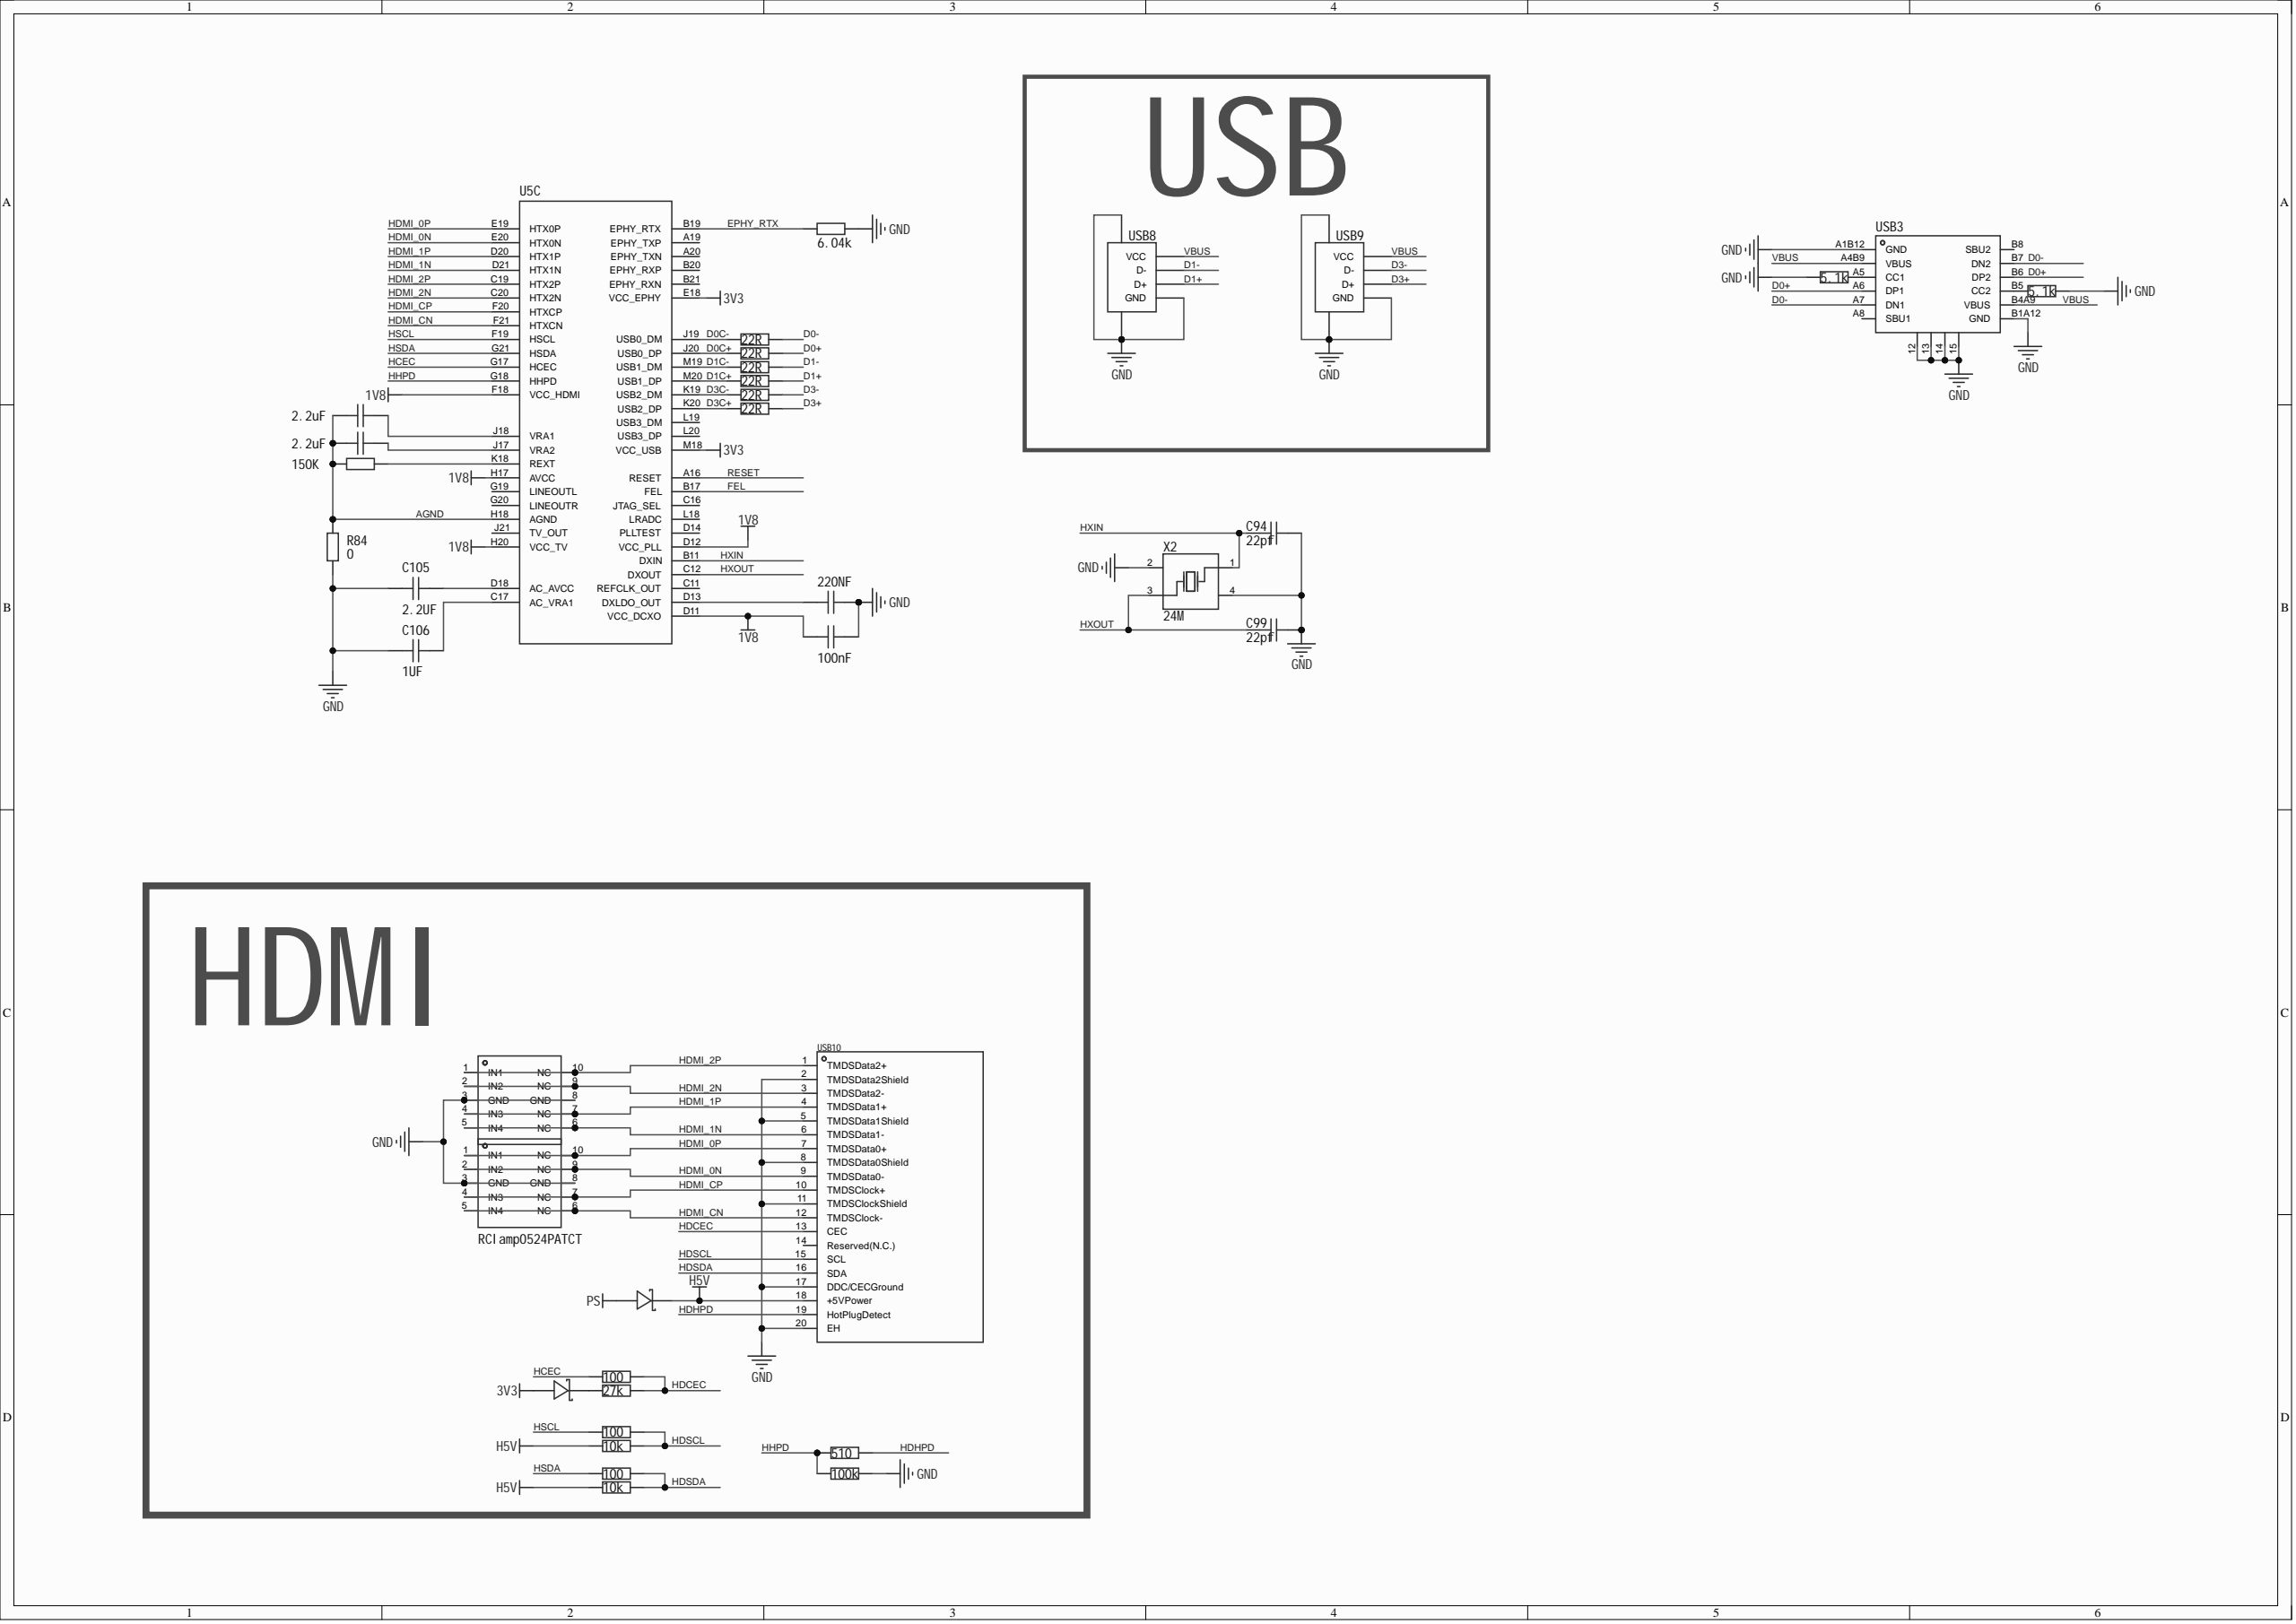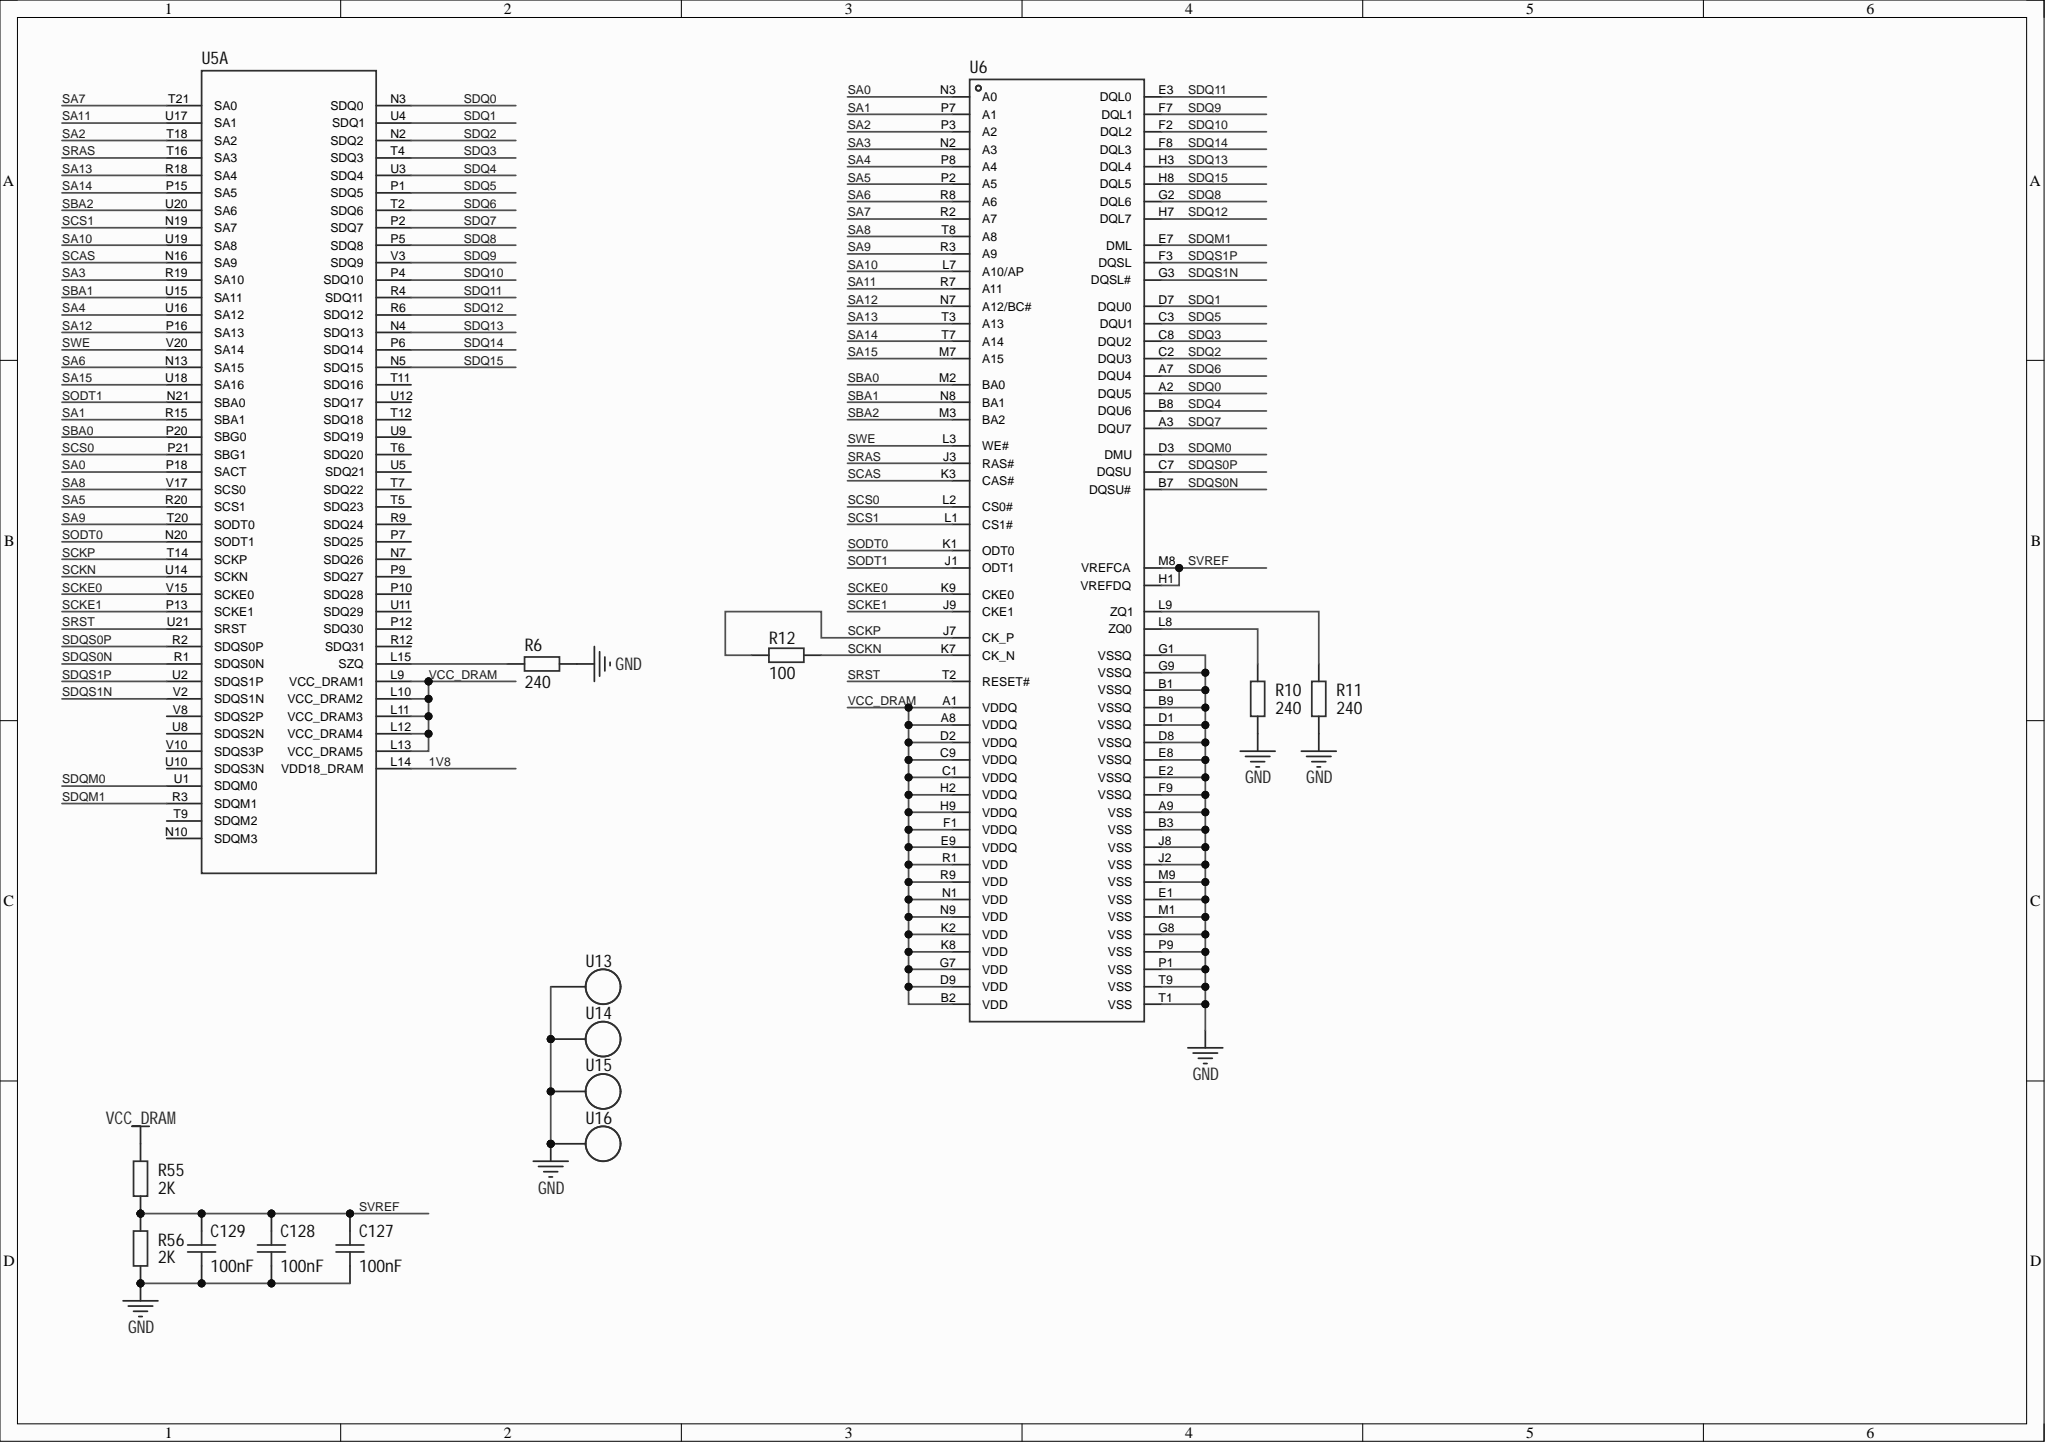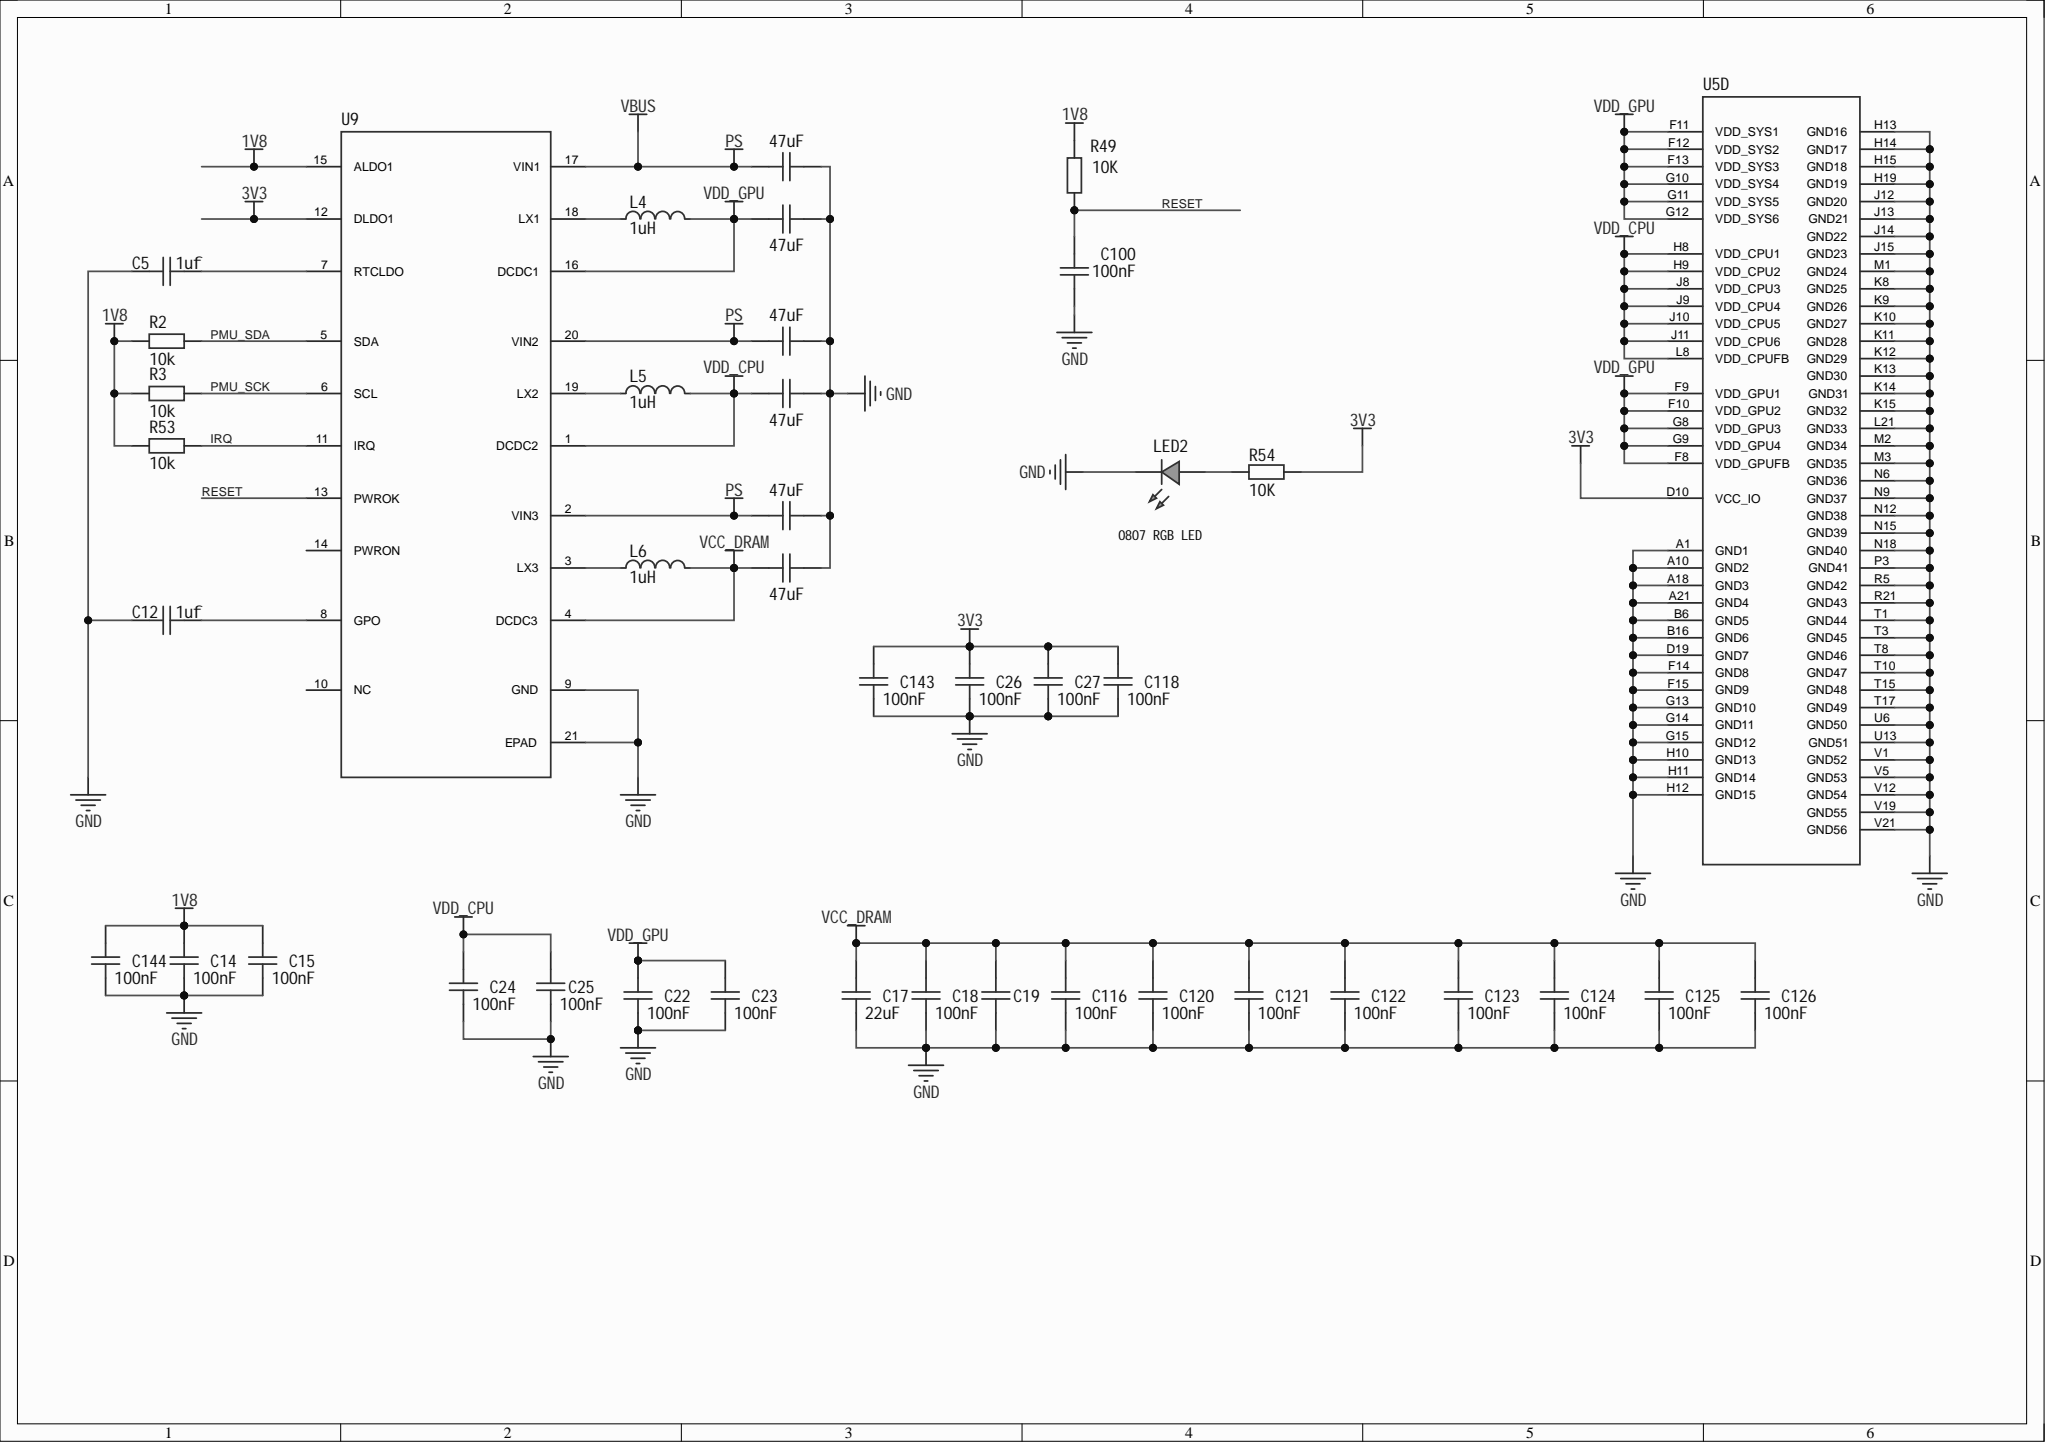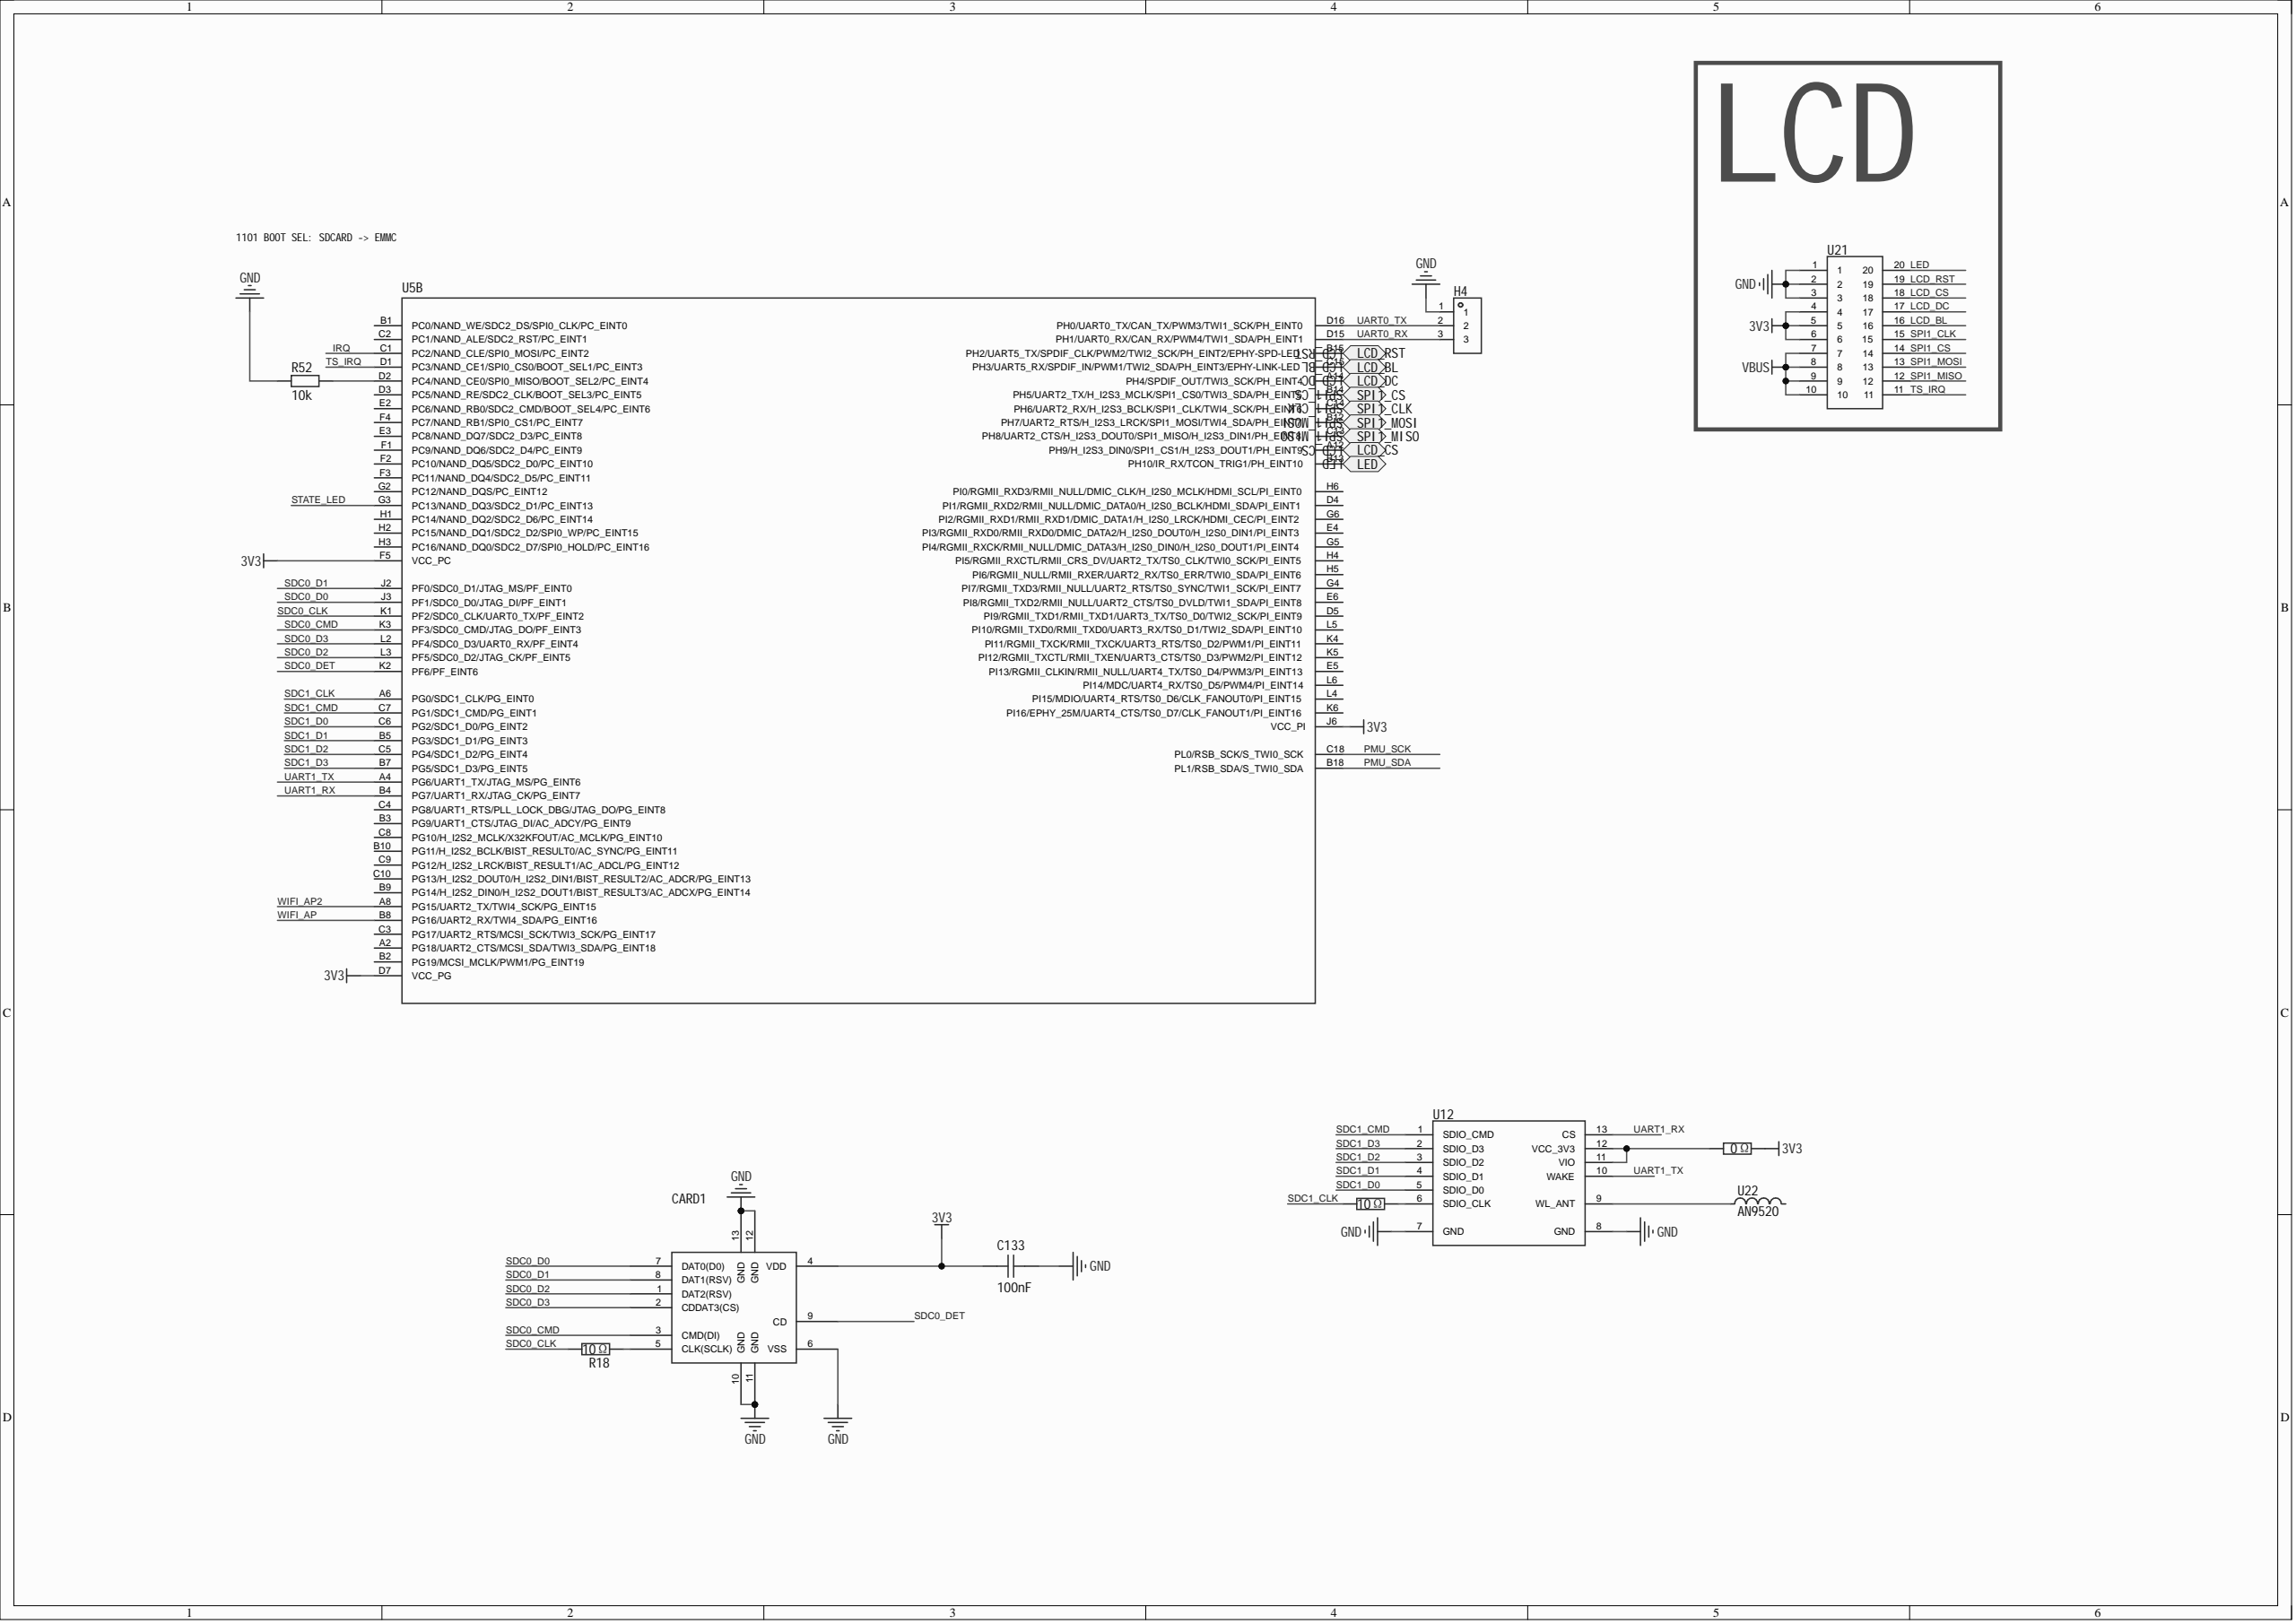Circuit board | Altium Designer | 102 parts | 149 nets
Bill of materials:
Comment,Description,Designator,Footprint,LibRef,Quantity
"","Capacitance:100nF;Tolerance:±10%;Rated voltage:16V;Temp. coefficient:X7R;","C5, C12, C14, C15, C17, C18, C19, C22, C23, C24, C25, C26, C27, C94, C99, C100, C116, C118, C120, C121, C122, C123, C124, C125, C126, C133, C143, C144","C0603 NSK","CAP_0402","28"
"2.2UF","","C105, C130, C131","C0603","CAP_0603","3"
"1UF","","C106","C0603","CAP_0603","1"
"220NF","","C108","C0603","CAP_0603","1"
"100nF","Capacitance:100nF;Tolerance:±10%;Rated voltage:50V;Material (temp. coefficient):X7R;","C127, C128, C129","C0402","CL05B104KB54PNC","3"
"100nF","","C132","C0603","CAP_0603","1"
"47uF","","C136, C137, C138, C139, C140, C141","C0805","CAP_0805","6"
"TF-015","Card connection mode:Push-push;Card type:MicroSD card (TF card);Connector type:Card socket;Body max height:-;Contact material:-;Contact plating:-;Operating temperature range:-;Soldering temperature (max):-;","CARD1","TF-SMD_TF-015","TF-015","1"
"","VBR=6V, Vc=15V, Ipp=5A","D24, D25","SLP2510P8_L2.5-W1.0-P0.50-BL","RClamp0524PATCT","2"
"","DC reverse voltage (Vr):40V;Average rectified current (Io):1A;Forward voltage drop (Vf):600mV@1A;","D26, D27","SOD-323_L1.8-W1.3-LS2.5-NSK","B5819WS","2"
"","","H4","HDR-TH_3P-P2.54-V-M","HDR-M_2.54_1x3P","1"
"1uH","Inductance:2.2uH;Tolerance:±20%;Rated current:2A;","L4, L5, L6","IND-SMD_L3.0-W3.0","SWPA3015S2R2MT","3"
"","","LED2","LED_0603","LED_0603-G","1"
"","","R2, R3, R43, R49, R52, R53, R70","R0603","Res_0402","7"
"","","R6","R0402-NSK_2","Res_0402","1"
"240","Resistor type:Thick film resistor;Resistance:200kΩ;Tolerance:±1%;Power:62.5mW;Max working voltage:50V;Temp. coefficient:±100ppm/?;","R10, R11","R0402","0402WGF2003TCE","2"
"100","Resistor type:Thick film resistor;Resistance:200kΩ;Tolerance:±1%;Power:62.5mW;Max working voltage:50V;Temp. coefficient:±100ppm/?;","R12","R0402","0402WGF2003TCE","1"
"10Ω","Tolerance:±1%;Temp. coefficient:±200ppm/;Power:1/16W;Resistance:10Ω;Max working voltage:50V;Operating temperature range:-55~+155;","R18, R86","R0603","0402WGF100JTCE","2"
"6.04k","Resistor type:Thick film resistor;Resistance:10kΩ;Tolerance:±1%;Power:100mW;","R26","R0603","0603WAF1002T5E","1"
"10K","","R54, R67, R88, R90, R117, R122","R0603","Res_0603","6"
"2K","Resistor type:Thick film resistor;Resistance:200kΩ;Tolerance:±1%;Power:62.5mW;Max working voltage:50V;Temp. coefficient:±100ppm/?;","R55, R56","R0402","0402WGF2003TCE","2"
"22R","","R66, R89, R91","R0603","Res_0603","3"
"150K","","R81","R0603","Res_0603","1"
"0","","R84","R0603","Res_0603","1"
"0Ω","Tolerance:±1%;Temp. coefficient:±200ppm/;Power:1/16W;Resistance:10Ω;Max working voltage:50V;Operating temperature range:-55~+155;","R87","R0603","0402WGF100JTCE","1"
"100","","R118, R121, R123","R0603","Res_0603","3"
"510","","R119","R0603","Res_0603","1"
"27k","","R120","R0603","Res_0603","1"
"100k","","R124","R0603","Res_0603","1"
"","","U5","BGA284P65B1200_1400H125","Allwinner_H616","1"
"","","U6","FBGA96","H5TQ4G63EFR-RDC","1"
"AXP313A","","U9","WQFN-20_L3.0-W3.0-P0.40-BL-EP","AXP1530","1"
"","","U12","WIFI模块","RTL8189ES模块","1"
"","","U13, U14, U15, U16","M3_HOLE","M3_HOLE","4"
"","","U21","BTB2X10","BTB2X10","1"
"AN9520","","U22","ANT-SMD_L9.5-W2.1","AN9520","1"
"","","USB3","USB-C-SMD_TYPEC-304-BCP16-1","TYPEC-304-BCP16","1"
"A/F board mount, type C, 10 (first two pins without curled edge), metal shell, LCP black glue=6.8","Connector type:Type-A;Standard:USB 2.0;Gender:Female;Ports:1;Contacts:4P;Rated current - power:-;","USB8, USB9","USB-A-SMD_C42496","A/F贴板 C款10前两脚无卷边铁壳LCP黑胶=6.8","2"
"HDMI 19PIN 043","Connector type:HDMI;Gender:Female;Total pins:19P;Rows:-;Mounting:Horizontal SMD;Rated current:300mA;Operating temperature range:-55℃~+85℃;","USB10","HDMI-SMD_HDMI-19PIN-043","HDMI 19PIN 043","1"
"24M","Crystal type:-;Frequency:-;Frequency tolerance:-;Frequency stability:-;Load capacitance:-;Operating temperature:-;","X2","OSC-SMD_4P-L2.0-W1.6-BL","SX32Y024000BC1T","1"
Netlist (Protel format):
[
C5
C0603 NSK




]
[
C12
C0603 NSK




]
[
C14
C0603 NSK




]
[
C15
C0603 NSK




]
[
C17
C0603 NSK




]
[
C18
C0603 NSK




]
[
C19
C0603 NSK




]
[
C22
C0603 NSK




]
[
C23
C0603 NSK




]
[
C24
C0603 NSK




]
[
C25
C0603 NSK




]
[
C26
C0603 NSK




]
[
C27
C0603 NSK




]
[
C94
C0603 NSK




]
[
C99
C0603 NSK




]
[
C100
C0603 NSK




]
[
C105
C0603
2.2UF



]
[
C106
C0603
1UF



]
[
C108
C0603
220NF



]
[
C116
C0603 NSK




]
[
C118
C0603 NSK




]
[
C120
C0603 NSK




]
[
C121
C0603 NSK




]
[
C122
C0603 NSK




]
[
C123
C0603 NSK




]
[
C124
C0603 NSK




]
[
C125
C0603 NSK




]
[
C126
C0603 NSK




]
[
C127
C0402
100nF



]
[
C128
C0402
100nF



]
[
C129
C0402
100nF



]
[
C130
C0603
2.2uF



]
[
C131
C0603
2.2uF



]
[
C132
C0603
100nF



]
[
C133
C0603 NSK




]
[
C136
C0805
47uF



]
[
C137
C0805
47uF



]
[
C138
C0805
47uF



]
[
C139
C0805
47uF



]
[
C140
C0805
47uF



]
[
C141
C0805
47uF



]
[
C143
C0603 NSK




]
[
C144
C0603 NSK




]
[
CARD1
TF-SMD_TF-015
TF-015



]
[
D24
SLP2510P8_L2.5-W1.0-P0.50-BL




]
[
D25
SLP2510P8_L2.5-W1.0-P0.50-BL




]
[
D26
SOD-323_L1.8-W1.3-LS2.5-NSK




]
[
D27
SOD-323_L1.8-W1.3-LS2.5-NSK




]
[
H4
HDR-TH_3P-P2.54-V-M




]
[
L4
IND-SMD_L3.0-W3.0
1uH



]
[
L5
IND-SMD_L3.0-W3.0
1uH



]
[
L6
IND-SMD_L3.0-W3.0
1uH



]
[
LED2
LED_0603




]
[
R2
R0603




]
[
R3
R0603




]
[
R6
R0402-NSK_2




]
[
R10
R0402
240



]
[
R11
R0402
240



]
[
R12
R0402
100



]
[
R18
R0603
10Ω



]
[
R26
R0603
6.04k



]
[
R43
R0603




]
[
R49
R0603




]
[
R52
R0603




]
[
R53
R0603




]
[
R54
R0603
10K



]
[
R55
R0402
2K



]
[
R56
R0402
2K



]
[
R66
R0603
22R



]
[
R67
R0603
10K



]
[
R70
R0603




]
[
R81
R0603
150K



]
[
R84
R0603
0



]
[
R86
R0603
10Ω



]
[
R87
R0603
0Ω



]
[
R88
R0603
10K



]
[
R89
R0603
22R



]
[
R90
R0603
10K



]
[
R91
R0603
22R



]
[
R117
R0603
10k



]
[
R118
R0603
100



]
[
R119
R0603
510



]
[
R120
R0603
27k



]
[
R121
R0603
100



]
[
R122
R0603
10k



]
[
R123
R0603
100



]
[
R124
R0603
100k



]
[
U5
BGA284P65B1200_1400H125




]
[
U6
FBGA96




]
[
U9
WQFN-20_L3.0-W3.0-P0.40-BL-EP
AXP313A



]
[
U12
WIFI模块




]
[
U13
M3_HOLE




]
[
U14
M3_HOLE




]
[
U15
M3_HOLE




]
[
U16
M3_HOLE




]
[
U21
BTB2X10




]
[
U22
ANT-SMD_L9.5-W2.1
AN9520



]
[
USB3
USB-C-SMD_TYPEC-304-BCP16-1




]
[
USB8
USB-A-SMD_C42496
A/F board mount, type C, 10 (first two pins without curled edge), metal shell, LCP black glue=6.8



]
[
USB9
USB-A-SMD_C42496
A/F board mount, type C, 10 (first two pins without curled edge), metal shell, LCP black glue=6.8



]
[
USB10
HDMI-SMD_HDMI-19PIN-043
HDMI 19PIN 043



]
[
X2
OSC-SMD_4P-L2.0-W1.6-BL
24M



]
(
VDD_GPU
C22-2
C23-2
C138-1
L4-2
U5-F8
U5-F9
U5-F10
U5-F11
U5-F12
U5-F13
U5-G8
U5-G9
U5-G10
U5-G11
U5-G12
U9-16
)
(
VDD_CPU
C24-2
C25-2
C136-1
L5-2
U5-H8
U5-H9
U5-J8
U5-J9
U5-J10
U5-J11
U5-L8
U9-1
)
(
VCC_DRAM
C17-2
C18-2
C19-2
C116-2
C120-2
C121-2
C122-2
C123-2
C124-2
C125-2
C126-2
C137-2
L6-2
R55-1
U5-L9
U5-L10
U5-L11
U5-L12
U5-L13
U6-A1
U6-A8
U6-B2
U6-C1
U6-C9
U6-D2
U6-D9
U6-E9
U6-F1
U6-G7
U6-H2
U6-H9
U6-K2
U6-K8
U6-N1
U6-N9
U6-R1
U6-R9
U9-4
)
(
VBUS
USB3-A4B9
USB3-B4A9
USB8-1
USB9-1
)
(
UART1_TX
U5-A4
U12-10
)
(
UART1_RX
U5-B4
U12-13
)
(
UART0_TX
H4-2
U5-D16
)
(
UART0_RX
H4-3
U5-D15
)
(
TS_IRQ
U5-D1
U21-11
)
(
SWE
U5-V20
U6-L3
)
(
SVREF
C127-2
C128-2
C129-2
R55-2
R56-1
U6-H1
U6-M8
)
(
SRST
U5-U21
U6-T2
)
(
SRAS
U5-T16
U6-J3
)
(
SPI1_MOSI
U5-B12
U21-13
)
(
SPI1_MISO
U5-C13
U21-12
)
(
SPI1_CS
U5-B14
U21-14
)
(
SPI1_CLK
U5-C14
U21-15
)
(
SODT1
U5-N21
U6-J1
)
(
SODT0
U5-N20
U6-K1
)
(
SDQS1P
U5-U2
U6-F3
)
(
SDQS1N
U5-V2
U6-G3
)
(
SDQS0P
U5-R2
U6-C7
)
(
SDQS0N
U5-R1
U6-B7
)
(
SDQM1
U5-R3
U6-E7
)
(
SDQM0
U5-U1
U6-D3
)
(
SDQ15
U5-N5
U6-H8
)
(
SDQ14
U5-P6
U6-F8
)
(
SDQ13
U5-N4
U6-H3
)
(
SDQ12
U5-R6
U6-H7
)
(
SDQ11
U5-R4
U6-E3
)
(
SDQ10
U5-P4
U6-F2
)
(
SDQ9
U5-V3
U6-F7
)
(
SDQ8
U5-P5
U6-G2
)
(
SDQ7
U5-P2
U6-A3
)
(
SDQ6
U5-T2
U6-A7
)
(
SDQ5
U5-P1
U6-C3
)
(
SDQ4
U5-U3
U6-B8
)
(
SDQ3
U5-T4
U6-C8
)
(
SDQ2
U5-N2
U6-C2
)
(
SDQ1
U5-U4
U6-D7
)
(
SDQ0
U5-N3
U6-A2
)
(
SDC1_D3
U5-B7
U12-2
)
(
SDC1_D2
U5-C5
U12-3
)
(
SDC1_D1
U5-B5
U12-4
)
(
SDC1_D0
U5-C6
U12-5
)
(
SDC1_CMD
U5-C7
U12-1
)
(
SDC1_CLK
R86-2
U5-A6
)
(
SDC0_DET
CARD1-9
U5-K2
)
(
SDC0_D3
CARD1-2
U5-L2
)
(
SDC0_D2
CARD1-1
U5-L3
)
(
SDC0_D1
CARD1-8
U5-J2
)
(
SDC0_D0
CARD1-7
U5-J3
)
(
SDC0_CMD
CARD1-3
U5-K3
)
(
SDC0_CLK
R18-1
U5-K1
)
(
SCS1
U5-N19
U6-L1
)
(
SCS0
U5-P21
U6-L2
)
(
SCKP
R12-2
U5-T14
U6-J7
)
(
SCKN
R12-1
U5-U14
U6-K7
)
(
SCKE1
U5-P13
U6-J9
)
(
SCKE0
U5-V15
U6-K9
)
(
SCAS
U5-N16
U6-K3
)
(
SBA2
U5-U20
U6-M3
)
(
SBA1
U5-U15
U6-N8
)
(
SBA0
U5-P20
U6-M2
)
(
SA15
U5-U18
U6-M7
)
(
SA14
U5-P15
U6-T7
)
(
SA13
U5-R18
U6-T3
)
(
SA12
U5-P16
U6-N7
)
(
SA11
U5-U17
U6-R7
)
(
SA10
U5-U19
U6-L7
)
(
SA9
U5-T20
U6-R3
)
(
SA8
U5-V17
U6-T8
)
(
SA7
U5-T21
U6-R2
)
(
SA6
U5-N13
U6-R8
)
(
SA5
U5-R20
U6-P2
)
(
SA4
U5-U16
U6-P8
)
(
SA3
U5-R19
U6-N2
)
(
SA2
U5-T18
U6-P3
)
(
SA1
U5-R15
U6-P7
)
(
SA0
U5-P18
U6-N3
)
(
RESET
C100-2
R49-1
U9-13
)
(
PS
C139-2
C140-2
C141-2
D26-2
U9-2
U9-17
U9-20
U21-7
U21-8
U21-9
U21-10
)
(
PMU_SDA
R2-2
U9-5
)
(
PMU_SCK
R3-2
U9-6
)
(
NetU12_9
U12-9
U22-1
)
(
NetR87_2
R87-2
U12-11
U12-12
)
(
NetR86_1
R86-1
U12-6
)
(
NetR81_2
R81-2
U5-K18
)
(
NetR70_2
R70-2
USB3-A5
)
(
NetR52_1
R52-1
U5-D2
)
(
NetR43_1
R43-1
USB3-B5
)
(
NetR11_2
R11-2
U6-L9
)
(
NetR10_2
R10-2
U6-L8
)
(
NetR6_1
R6-1
U5-L15
)
(
NetLED2_2
LED2-2
R54-1
)
(
NetL6_1
L6-1
U9-3
)
(
NetL5_1
L5-1
U9-19
)
(
NetL4_1
L4-1
U9-18
)
(
NetD27_1
D27-1
R120-1
)
(
NetCARD1_5
CARD1-5
R18-2
)
(
NetC131_2
C131-2
U5-J17
)
(
NetC130_2
C130-2
U5-J18
)
(
NetC108_1
C108-1
U5-D13
)
(
NetC106_2
C106-2
U5-C17
)
(
NetC105_2
C105-2
U5-D18
)
(
NetC12_2
C12-2
U9-8
)
(
NetC5_2
C5-2
U9-7
)
(
LED
U5-B13
U21-20
)
(
LCD_RST
U5-B15
U21-19
)
(
LCD_DC
U5-A14
U21-17
)
(
LCD_CS
U5-A12
U21-18
)
(
LCD_BL
U5-C15
U21-16
)
(
IRQ
R53-2
U9-11
)
(
HXOUT
C99-1
U5-C12
X2-3
)
(
HXIN
C94-1
U5-B11
X2-1
)
(
HSDA
R118-1
U5-G21
)
(
HSCL
R123-1
U5-F19
)
(
HHPD
R119-1
R124-1
U5-G18
)
(
HDSDA
R117-2
R118-2
USB10-16
)
(
HDSCL
R122-2
R123-2
USB10-15
)
(
HDMI_CP
D25-4
D25-7
U5-F20
USB10-10
)
(
HDMI_CN
D25-5
D25-6
U5-F21
USB10-12
)
(
HDMI_2P
D24-1
D24-10
U5-C19
USB10-1
)
(
HDMI_2N
D24-2
D24-9
U5-C20
USB10-3
)
(
HDMI_1P
D24-4
D24-7
U5-D20
USB10-4
)
(
HDMI_1N
D24-5
D24-6
U5-D21
USB10-6
)
(
HDMI_0P
D25-1
D25-10
U5-E19
USB10-7
)
(
HDMI_0N
D25-2
D25-9
U5-E20
USB10-9
)
(
HDHPD
R119-2
USB10-19
)
(
HDCEC
R120-2
R121-2
USB10-13
)
(
HCEC
R121-1
U5-G17
)
(
H5V
D26-1
R117-1
R122-1
USB10-18
)
(
GND
C5-1
C12-1
C14-1
C15-1
C17-1
C18-1
C19-1
C22-1
C23-1
C24-1
C25-1
C26-1
C27-1
C94-2
C99-2
C100-1
C105-1
C106-1
C108-2
C116-1
C118-1
C120-1
C121-1
C122-1
C123-1
C124-1
C125-1
C126-1
C127-1
C128-1
C129-1
C132-2
C133-1
C136-2
C137-1
C138-2
C139-1
C140-1
C141-1
C143-1
C144-1
CARD1-6
CARD1-10
CARD1-11
CARD1-12
CARD1-13
D24-3
D24-8
D25-3
D25-8
H4-1
LED2-1
R6-2
R10-1
R11-1
R26-2
R43-2
R52-2
R56-2
R70-1
R84-1
R124-2
U5-A1
U5-A10
U5-A18
U5-A21
U5-B6
U5-B16
U5-D19
U5-F14
U5-F15
U5-G13
U5-G14
U5-G15
U5-H10
U5-H11
U5-H12
U5-H13
U5-H14
U5-H15
U5-H19
U5-J12
U5-J13
U5-J14
U5-J15
U5-K8
U5-K9
U5-K10
U5-K11
U5-K12
U5-K13
U5-K14
U5-K15
U5-L21
U5-M1
U5-M2
U5-M3
U5-N6
U5-N9
U5-N12
U5-N15
U5-N18
U5-P3
U5-R5
U5-R21
U5-T1
U5-T3
U5-T8
U5-T10
U5-T15
U5-T17
U5-U6
U5-U13
U5-V1
U5-V5
U5-V12
U5-V19
U5-V21
U6-A9
U6-B1
U6-B3
U6-B9
U6-D1
U6-D8
U6-E1
U6-E2
U6-E8
U6-F9
U6-G1
U6-G8
U6-G9
U6-J2
U6-J8
U6-M1
U6-M9
U6-P1
U6-P9
U6-T1
U6-T9
U9-9
U9-21
U12-7
U12-8
U13-1
U14-1
U15-1
U16-1
U21-1
U21-2
U21-3
USB3-12
USB3-13
USB3-14
USB3-15
USB3-A1B12
USB3-B1A12
USB8-4
USB8-5
USB8-6
USB9-4
USB9-5
USB9-6
USB10-2
USB10-5
USB10-8
USB10-11
USB10-17
USB10-20
X2-2
X2-4
)
(
EPHY_RTX
R26-1
U5-B19
)
(
D3C-
R91-1
U5-K19
)
(
D3C+
R90-1
U5-K20
)
(
D3-
R91-2
USB9-2
)
(
D3+
R90-2
USB9-3
)
(
D1C-
R89-1
U5-M19
)
(
D1C+
R88-1
U5-M20
)
(
D1-
R89-2
USB8-2
)
(
D1+
R88-2
USB8-3
)
(
D0C-
R66-1
U5-J19
)
(
D0C+
R67-1
U5-J20
)
(
D0-
R66-2
USB3-A7
USB3-B7
)
(
D0+
R67-2
USB3-A6
USB3-B6
)
(
AGND
C130-1
C131-1
R81-1
R84-2
U5-H18
)
(
3V3
C26-2
C27-2
C118-2
C133-2
C143-2
CARD1-4
D27-2
R54-2
R87-1
U5-D7
U5-D10
U5-E18
U5-F5
U5-J6
U5-M18
U9-12
U21-4
U21-5
U21-6
)
(
1V8
C14-2
C15-2
C132-1
C144-2
R2-1
R3-1
R49-2
R53-1
U5-D11
U5-D12
U5-F18
U5-H17
U5-H20
U9-15
)